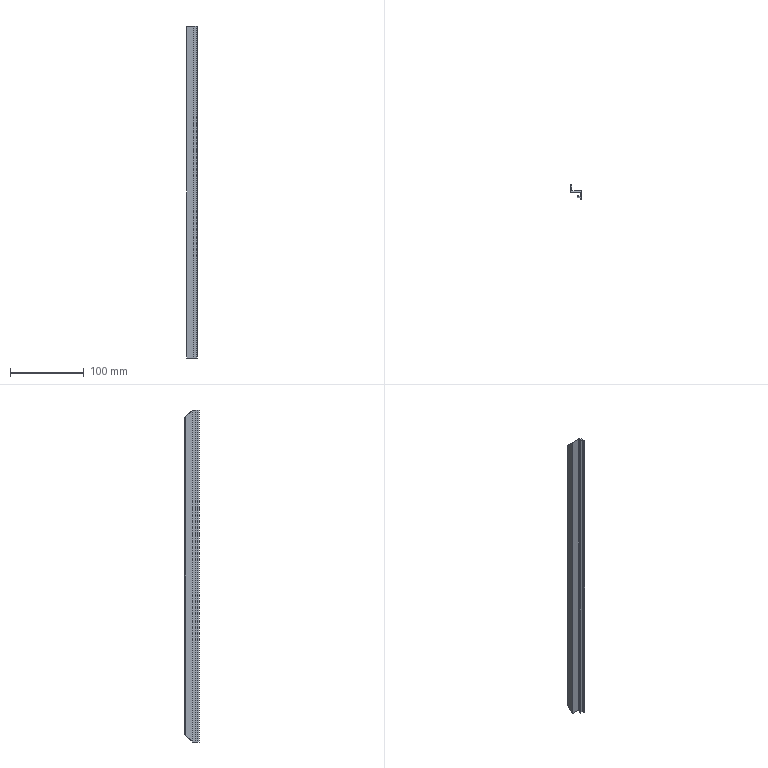Part | NX | features BREP 1 | 1 solid | 19 faces | box 14.9 x 19.1 x 450 mm | volume 31786 mm3 | plane 16 | cylinder 3 | commonest cylinder face diameters 1 x2 2 x1
STEP:
#1=CARTESIAN_POINT('',(12.9,-1.,223.5));
#2=VERTEX_POINT('',#1);
#3=CARTESIAN_POINT('',(12.9,-1.,-223.5));
#4=VERTEX_POINT('',#3);
#5=CARTESIAN_POINT('',(12.9,-1.,225.));
#6=DIRECTION('',(0.,0.,-1.));
#7=VECTOR('',#6,1000.);
#8=LINE('',#5,#7);
#9=EDGE_CURVE('',#2,#4,#8,.T.);
#10=ORIENTED_EDGE('',*,*,#9,.T.);
#11=CARTESIAN_POINT('',(12.4,-0.5,-223.));
#12=VERTEX_POINT('',#11);
#13=CARTESIAN_POINT('',(12.9,-1.,-223.5));
#14=CARTESIAN_POINT('',(12.9,-0.7071,-223.207));
#15=CARTESIAN_POINT('',(12.693,-0.5,-223.));
#16=CARTESIAN_POINT('',(12.4,-0.5,-223.));
#17=(BOUNDED_CURVE()B_SPLINE_CURVE(3,(#13,#14,#15,#16),.UNSPECIFIED.,.F.,.F.)B_SPLINE_CURVE_WITH_KNOTS((4,4),(1.571,3.142),.UNSPECIFIED.)CURVE()GEOMETRIC_REPRESENTATION_ITEM()RATIONAL_B_SPLINE_CURVE((1.,0.8047,0.8047,1.))REPRESENTATION_ITEM(''));
#18=EDGE_CURVE('',#4,#12,#17,.T.);
#19=ORIENTED_EDGE('',*,*,#18,.T.);
#20=CARTESIAN_POINT('',(12.4,-0.5,223.));
#21=VERTEX_POINT('',#20);
#22=CARTESIAN_POINT('',(12.4,-0.5,225.));
#23=DIRECTION('',(0.,0.,-1.));
#24=VECTOR('',#23,1000.);
#25=LINE('',#22,#24);
#26=EDGE_CURVE('',#21,#12,#25,.T.);
#27=ORIENTED_EDGE('',*,*,#26,.F.);
#28=CARTESIAN_POINT('',(12.4,-0.5,223.));
#29=CARTESIAN_POINT('',(12.693,-0.5,223.));
#30=CARTESIAN_POINT('',(12.9,-0.7071,223.207));
#31=CARTESIAN_POINT('',(12.9,-1.,223.5));
#32=(BOUNDED_CURVE()B_SPLINE_CURVE(3,(#28,#29,#30,#31),.UNSPECIFIED.,.F.,.F.)B_SPLINE_CURVE_WITH_KNOTS((4,4),(0.,1.571),.UNSPECIFIED.)CURVE()GEOMETRIC_REPRESENTATION_ITEM()RATIONAL_B_SPLINE_CURVE((1.,0.8047,0.8047,1.))REPRESENTATION_ITEM(''));
#33=EDGE_CURVE('',#21,#2,#32,.T.);
#34=ORIENTED_EDGE('',*,*,#33,.T.);
#35=EDGE_LOOP('',(#10,#19,#27,#34));
#36=FACE_BOUND('',#35,.T.);
#37=CARTESIAN_POINT('',(12.4,-1.,225.));
#38=DIRECTION('',(0.,0.,-1.));
#39=DIRECTION('',(-1.,0.,0.));
#40=AXIS2_PLACEMENT_3D('',#37,#38,#39);
#41=CYLINDRICAL_SURFACE('',#40,0.5);
#42=ADVANCED_FACE('',(#36),#41,.T.);
#43=ORIENTED_EDGE('',*,*,#26,.T.);
#44=CARTESIAN_POINT('',(0.,-0.5,-223.));
#45=VERTEX_POINT('',#44);
#46=CARTESIAN_POINT('',(0.,-0.5,-223.));
#47=DIRECTION('',(-1.,0.,0.));
#48=VECTOR('',#47,1000.);
#49=LINE('',#46,#48);
#50=EDGE_CURVE('',#12,#45,#49,.T.);
#51=ORIENTED_EDGE('',*,*,#50,.T.);
#52=CARTESIAN_POINT('',(0.,-0.5,223.));
#53=VERTEX_POINT('',#52);
#54=CARTESIAN_POINT('',(0.,-0.5,225.));
#55=DIRECTION('',(0.,0.,-1.));
#56=VECTOR('',#55,1000.);
#57=LINE('',#54,#56);
#58=EDGE_CURVE('',#53,#45,#57,.T.);
#59=ORIENTED_EDGE('',*,*,#58,.F.);
#60=CARTESIAN_POINT('',(12.4,-0.5,223.));
#61=DIRECTION('',(1.,0.,0.));
#62=VECTOR('',#61,1000.);
#63=LINE('',#60,#62);
#64=EDGE_CURVE('',#53,#21,#63,.T.);
#65=ORIENTED_EDGE('',*,*,#64,.T.);
#66=EDGE_LOOP('',(#43,#51,#59,#65));
#67=FACE_BOUND('',#66,.T.);
#68=CARTESIAN_POINT('',(12.4,-0.5,225.));
#69=DIRECTION('',(0.,-1.,0.));
#70=DIRECTION('',(0.,0.,-1.));
#71=AXIS2_PLACEMENT_3D('',#68,#69,#70);
#72=PLANE('',#71);
#73=ADVANCED_FACE('',(#67),#72,.F.);
#74=ORIENTED_EDGE('',*,*,#58,.T.);
#75=CARTESIAN_POINT('',(0.,7.5,-215.));
#76=VERTEX_POINT('',#75);
#77=CARTESIAN_POINT('',(0.,7.5,-215.));
#78=DIRECTION('',(0.,0.7071,0.7071));
#79=VECTOR('',#78,1000.);
#80=LINE('',#77,#79);
#81=EDGE_CURVE('',#45,#76,#80,.T.);
#82=ORIENTED_EDGE('',*,*,#81,.T.);
#83=CARTESIAN_POINT('',(0.,7.5,215.));
#84=VERTEX_POINT('',#83);
#85=CARTESIAN_POINT('',(0.,7.5,225.));
#86=DIRECTION('',(0.,0.,-1.));
#87=VECTOR('',#86,1000.);
#88=LINE('',#85,#87);
#89=EDGE_CURVE('',#84,#76,#88,.T.);
#90=ORIENTED_EDGE('',*,*,#89,.F.);
#91=CARTESIAN_POINT('',(0.,-2.5,225.));
#92=DIRECTION('',(0.,-0.7071,0.7071));
#93=VECTOR('',#92,1000.);
#94=LINE('',#91,#93);
#95=EDGE_CURVE('',#84,#53,#94,.T.);
#96=ORIENTED_EDGE('',*,*,#95,.T.);
#97=EDGE_LOOP('',(#74,#82,#90,#96));
#98=FACE_BOUND('',#97,.T.);
#99=CARTESIAN_POINT('',(0.,-0.5,225.));
#100=DIRECTION('',(-1.,0.,0.));
#101=DIRECTION('',(0.,0.,1.));
#102=AXIS2_PLACEMENT_3D('',#99,#100,#101);
#103=PLANE('',#102);
#104=ADVANCED_FACE('',(#98),#103,.F.);
#105=ORIENTED_EDGE('',*,*,#89,.T.);
#106=CARTESIAN_POINT('',(-1.,7.5,-215.));
#107=VERTEX_POINT('',#106);
#108=CARTESIAN_POINT('',(0.,7.5,-215.));
#109=DIRECTION('',(-1.,0.,0.));
#110=VECTOR('',#109,1000.);
#111=LINE('',#108,#110);
#112=EDGE_CURVE('',#76,#107,#111,.T.);
#113=ORIENTED_EDGE('',*,*,#112,.T.);
#114=CARTESIAN_POINT('',(-1.,7.5,215.));
#115=VERTEX_POINT('',#114);
#116=CARTESIAN_POINT('',(-1.,7.5,225.));
#117=DIRECTION('',(0.,0.,-1.));
#118=VECTOR('',#117,1000.);
#119=LINE('',#116,#118);
#120=EDGE_CURVE('',#115,#107,#119,.T.);
#121=ORIENTED_EDGE('',*,*,#120,.F.);
#122=CARTESIAN_POINT('',(0.,7.5,215.));
#123=DIRECTION('',(1.,0.,0.));
#124=VECTOR('',#123,1000.);
#125=LINE('',#122,#124);
#126=EDGE_CURVE('',#115,#84,#125,.T.);
#127=ORIENTED_EDGE('',*,*,#126,.T.);
#128=EDGE_LOOP('',(#105,#113,#121,#127));
#129=FACE_BOUND('',#128,.T.);
#130=CARTESIAN_POINT('',(0.,7.5,225.));
#131=DIRECTION('',(0.,-1.,0.));
#132=DIRECTION('',(0.,0.,-1.));
#133=AXIS2_PLACEMENT_3D('',#130,#131,#132);
#134=PLANE('',#133);
#135=ADVANCED_FACE('',(#129),#134,.F.);
#136=ORIENTED_EDGE('',*,*,#120,.T.);
#137=CARTESIAN_POINT('',(-2.,6.5,-216.));
#138=VERTEX_POINT('',#137);
#139=CARTESIAN_POINT('',(-1.,7.5,-215.));
#140=CARTESIAN_POINT('',(-1.586,7.5,-215.));
#141=CARTESIAN_POINT('',(-2.,7.086,-215.414));
#142=CARTESIAN_POINT('',(-2.,6.5,-216.));
#143=(BOUNDED_CURVE()B_SPLINE_CURVE(3,(#139,#140,#141,#142),.UNSPECIFIED.,.F.,.F.)B_SPLINE_CURVE_WITH_KNOTS((4,4),(3.142,4.712),.UNSPECIFIED.)CURVE()GEOMETRIC_REPRESENTATION_ITEM()RATIONAL_B_SPLINE_CURVE((1.,0.8047,0.8047,1.))REPRESENTATION_ITEM(''));
#144=EDGE_CURVE('',#107,#138,#143,.T.);
#145=ORIENTED_EDGE('',*,*,#144,.T.);
#146=CARTESIAN_POINT('',(-2.,6.5,216.));
#147=VERTEX_POINT('',#146);
#148=CARTESIAN_POINT('',(-2.,6.5,225.));
#149=DIRECTION('',(0.,0.,-1.));
#150=VECTOR('',#149,1000.);
#151=LINE('',#148,#150);
#152=EDGE_CURVE('',#147,#138,#151,.T.);
#153=ORIENTED_EDGE('',*,*,#152,.F.);
#154=CARTESIAN_POINT('',(-2.,6.5,216.));
#155=CARTESIAN_POINT('',(-2.,7.086,215.414));
#156=CARTESIAN_POINT('',(-1.586,7.5,215.));
#157=CARTESIAN_POINT('',(-1.,7.5,215.));
#158=(BOUNDED_CURVE()B_SPLINE_CURVE(3,(#154,#155,#156,#157),.UNSPECIFIED.,.F.,.F.)B_SPLINE_CURVE_WITH_KNOTS((4,4),(4.712,6.283),.UNSPECIFIED.)CURVE()GEOMETRIC_REPRESENTATION_ITEM()RATIONAL_B_SPLINE_CURVE((1.,0.8047,0.8047,1.))REPRESENTATION_ITEM(''));
#159=EDGE_CURVE('',#147,#115,#158,.T.);
#160=ORIENTED_EDGE('',*,*,#159,.T.);
#161=EDGE_LOOP('',(#136,#145,#153,#160));
#162=FACE_BOUND('',#161,.T.);
#163=CARTESIAN_POINT('',(-1.,6.5,225.));
#164=DIRECTION('',(0.,0.,-1.));
#165=DIRECTION('',(-1.,0.,0.));
#166=AXIS2_PLACEMENT_3D('',#163,#164,#165);
#167=CYLINDRICAL_SURFACE('',#166,1.);
#168=ADVANCED_FACE('',(#162),#167,.T.);
#169=ORIENTED_EDGE('',*,*,#152,.T.);
#170=CARTESIAN_POINT('',(-2.,-2.5,-225.));
#171=VERTEX_POINT('',#170);
#172=CARTESIAN_POINT('',(-2.,7.5,-215.));
#173=DIRECTION('',(0.,-0.7071,-0.7071));
#174=VECTOR('',#173,1000.);
#175=LINE('',#172,#174);
#176=EDGE_CURVE('',#138,#171,#175,.T.);
#177=ORIENTED_EDGE('',*,*,#176,.T.);
#178=CARTESIAN_POINT('',(-2.,-2.5,225.));
#179=VERTEX_POINT('',#178);
#180=CARTESIAN_POINT('',(-2.,-2.5,225.));
#181=DIRECTION('',(0.,0.,-1.));
#182=VECTOR('',#181,1000.);
#183=LINE('',#180,#182);
#184=EDGE_CURVE('',#179,#171,#183,.T.);
#185=ORIENTED_EDGE('',*,*,#184,.F.);
#186=CARTESIAN_POINT('',(-2.,-2.5,225.));
#187=DIRECTION('',(0.,0.7071,-0.7071));
#188=VECTOR('',#187,1000.);
#189=LINE('',#186,#188);
#190=EDGE_CURVE('',#179,#147,#189,.T.);
#191=ORIENTED_EDGE('',*,*,#190,.T.);
#192=EDGE_LOOP('',(#169,#177,#185,#191));
#193=FACE_BOUND('',#192,.T.);
#194=CARTESIAN_POINT('',(-2.,6.5,225.));
#195=DIRECTION('',(1.,0.,0.));
#196=DIRECTION('',(0.,1.,0.));
#197=AXIS2_PLACEMENT_3D('',#194,#195,#196);
#198=PLANE('',#197);
#199=ADVANCED_FACE('',(#193),#198,.F.);
#200=CARTESIAN_POINT('',(10.4,-2.5,-225.));
#201=VERTEX_POINT('',#200);
#202=CARTESIAN_POINT('',(-2.,-2.5,-225.));
#203=DIRECTION('',(1.,0.,0.));
#204=VECTOR('',#203,1000.);
#205=LINE('',#202,#204);
#206=EDGE_CURVE('',#171,#201,#205,.T.);
#207=ORIENTED_EDGE('',*,*,#206,.T.);
#208=CARTESIAN_POINT('',(10.4,-2.5,225.));
#209=VERTEX_POINT('',#208);
#210=CARTESIAN_POINT('',(10.4,-2.5,225.));
#211=DIRECTION('',(0.,0.,-1.));
#212=VECTOR('',#211,1000.);
#213=LINE('',#210,#212);
#214=EDGE_CURVE('',#209,#201,#213,.T.);
#215=ORIENTED_EDGE('',*,*,#214,.F.);
#216=CARTESIAN_POINT('',(-2.,-2.5,225.));
#217=DIRECTION('',(1.,0.,0.));
#218=VECTOR('',#217,1000.);
#219=LINE('',#216,#218);
#220=EDGE_CURVE('',#179,#209,#219,.T.);
#221=ORIENTED_EDGE('',*,*,#220,.F.);
#222=ORIENTED_EDGE('',*,*,#184,.T.);
#223=EDGE_LOOP('',(#207,#215,#221,#222));
#224=FACE_BOUND('',#223,.T.);
#225=CARTESIAN_POINT('',(-2.,-2.5,225.));
#226=DIRECTION('',(0.,1.,0.));
#227=DIRECTION('',(1.,0.,0.));
#228=AXIS2_PLACEMENT_3D('',#225,#226,#227);
#229=PLANE('',#228);
#230=ADVANCED_FACE('',(#224),#229,.F.);
#231=CARTESIAN_POINT('',(10.9,-3.,-225.));
#232=VERTEX_POINT('',#231);
#233=CARTESIAN_POINT('',(10.4,-3.,-225.));
#234=DIRECTION('',(0.,0.,-1.));
#235=DIRECTION('',(1.,0.,0.));
#236=AXIS2_PLACEMENT_3D('',#233,#234,#235);
#237=CIRCLE('',#236,0.5);
#238=EDGE_CURVE('',#201,#232,#237,.T.);
#239=ORIENTED_EDGE('',*,*,#238,.T.);
#240=CARTESIAN_POINT('',(10.9,-3.,225.));
#241=VERTEX_POINT('',#240);
#242=CARTESIAN_POINT('',(10.9,-3.,225.));
#243=DIRECTION('',(0.,0.,-1.));
#244=VECTOR('',#243,1000.);
#245=LINE('',#242,#244);
#246=EDGE_CURVE('',#241,#232,#245,.T.);
#247=ORIENTED_EDGE('',*,*,#246,.F.);
#248=CARTESIAN_POINT('',(10.4,-3.,225.));
#249=DIRECTION('',(0.,0.,-1.));
#250=DIRECTION('',(1.,0.,0.));
#251=AXIS2_PLACEMENT_3D('',#248,#249,#250);
#252=CIRCLE('',#251,0.5);
#253=EDGE_CURVE('',#209,#241,#252,.T.);
#254=ORIENTED_EDGE('',*,*,#253,.F.);
#255=ORIENTED_EDGE('',*,*,#214,.T.);
#256=EDGE_LOOP('',(#239,#247,#254,#255));
#257=FACE_BOUND('',#256,.T.);
#258=CARTESIAN_POINT('',(10.4,-3.,225.));
#259=DIRECTION('',(0.,0.,-1.));
#260=DIRECTION('',(-1.,0.,0.));
#261=AXIS2_PLACEMENT_3D('',#258,#259,#260);
#262=CYLINDRICAL_SURFACE('',#261,0.5);
#263=ADVANCED_FACE('',(#257),#262,.F.);
#264=CARTESIAN_POINT('',(10.9,-7.2,-225.));
#265=VERTEX_POINT('',#264);
#266=CARTESIAN_POINT('',(10.9,-3.,-225.));
#267=DIRECTION('',(0.,-1.,0.));
#268=VECTOR('',#267,1000.);
#269=LINE('',#266,#268);
#270=EDGE_CURVE('',#232,#265,#269,.T.);
#271=ORIENTED_EDGE('',*,*,#270,.T.);
#272=CARTESIAN_POINT('',(10.9,-7.2,225.));
#273=VERTEX_POINT('',#272);
#274=CARTESIAN_POINT('',(10.9,-7.2,225.));
#275=DIRECTION('',(0.,0.,-1.));
#276=VECTOR('',#275,1000.);
#277=LINE('',#274,#276);
#278=EDGE_CURVE('',#273,#265,#277,.T.);
#279=ORIENTED_EDGE('',*,*,#278,.F.);
#280=CARTESIAN_POINT('',(10.9,-3.,225.));
#281=DIRECTION('',(0.,-1.,0.));
#282=VECTOR('',#281,1000.);
#283=LINE('',#280,#282);
#284=EDGE_CURVE('',#241,#273,#283,.T.);
#285=ORIENTED_EDGE('',*,*,#284,.F.);
#286=ORIENTED_EDGE('',*,*,#246,.T.);
#287=EDGE_LOOP('',(#271,#279,#285,#286));
#288=FACE_BOUND('',#287,.T.);
#289=CARTESIAN_POINT('',(10.9,-3.,225.));
#290=DIRECTION('',(1.,0.,0.));
#291=DIRECTION('',(0.,1.,0.));
#292=AXIS2_PLACEMENT_3D('',#289,#290,#291);
#293=PLANE('',#292);
#294=ADVANCED_FACE('',(#288),#293,.F.);
#295=CARTESIAN_POINT('',(7.2,-7.2,-225.));
#296=VERTEX_POINT('',#295);
#297=CARTESIAN_POINT('',(10.9,-7.2,-225.));
#298=DIRECTION('',(-1.,0.,0.));
#299=VECTOR('',#298,1000.);
#300=LINE('',#297,#299);
#301=EDGE_CURVE('',#265,#296,#300,.T.);
#302=ORIENTED_EDGE('',*,*,#301,.T.);
#303=CARTESIAN_POINT('',(7.2,-7.2,225.));
#304=VERTEX_POINT('',#303);
#305=CARTESIAN_POINT('',(7.2,-7.2,225.));
#306=DIRECTION('',(0.,0.,-1.));
#307=VECTOR('',#306,1000.);
#308=LINE('',#305,#307);
#309=EDGE_CURVE('',#304,#296,#308,.T.);
#310=ORIENTED_EDGE('',*,*,#309,.F.);
#311=CARTESIAN_POINT('',(10.9,-7.2,225.));
#312=DIRECTION('',(-1.,0.,0.));
#313=VECTOR('',#312,1000.);
#314=LINE('',#311,#313);
#315=EDGE_CURVE('',#273,#304,#314,.T.);
#316=ORIENTED_EDGE('',*,*,#315,.F.);
#317=ORIENTED_EDGE('',*,*,#278,.T.);
#318=EDGE_LOOP('',(#302,#310,#316,#317));
#319=FACE_BOUND('',#318,.T.);
#320=CARTESIAN_POINT('',(10.9,-7.2,225.));
#321=DIRECTION('',(0.,-1.,0.));
#322=DIRECTION('',(0.,0.,-1.));
#323=AXIS2_PLACEMENT_3D('',#320,#321,#322);
#324=PLANE('',#323);
#325=ADVANCED_FACE('',(#319),#324,.F.);
#326=CARTESIAN_POINT('',(7.2,-9.2,-225.));
#327=VERTEX_POINT('',#326);
#328=CARTESIAN_POINT('',(7.2,-7.2,-225.));
#329=DIRECTION('',(0.,-1.,0.));
#330=VECTOR('',#329,1000.);
#331=LINE('',#328,#330);
#332=EDGE_CURVE('',#296,#327,#331,.T.);
#333=ORIENTED_EDGE('',*,*,#332,.T.);
#334=CARTESIAN_POINT('',(7.2,-9.2,225.));
#335=VERTEX_POINT('',#334);
#336=CARTESIAN_POINT('',(7.2,-9.2,225.));
#337=DIRECTION('',(0.,0.,-1.));
#338=VECTOR('',#337,1000.);
#339=LINE('',#336,#338);
#340=EDGE_CURVE('',#335,#327,#339,.T.);
#341=ORIENTED_EDGE('',*,*,#340,.F.);
#342=CARTESIAN_POINT('',(7.2,-7.2,225.));
#343=DIRECTION('',(0.,-1.,0.));
#344=VECTOR('',#343,1000.);
#345=LINE('',#342,#344);
#346=EDGE_CURVE('',#304,#335,#345,.T.);
#347=ORIENTED_EDGE('',*,*,#346,.F.);
#348=ORIENTED_EDGE('',*,*,#309,.T.);
#349=EDGE_LOOP('',(#333,#341,#347,#348));
#350=FACE_BOUND('',#349,.T.);
#351=CARTESIAN_POINT('',(7.2,-7.2,225.));
#352=DIRECTION('',(1.,0.,0.));
#353=DIRECTION('',(0.,1.,0.));
#354=AXIS2_PLACEMENT_3D('',#351,#352,#353);
#355=PLANE('',#354);
#356=ADVANCED_FACE('',(#350),#355,.F.);
#357=CARTESIAN_POINT('',(10.9,-9.2,-225.));
#358=VERTEX_POINT('',#357);
#359=CARTESIAN_POINT('',(7.2,-9.2,-225.));
#360=DIRECTION('',(1.,0.,0.));
#361=VECTOR('',#360,1000.);
#362=LINE('',#359,#361);
#363=EDGE_CURVE('',#327,#358,#362,.T.);
#364=ORIENTED_EDGE('',*,*,#363,.T.);
#365=CARTESIAN_POINT('',(10.9,-9.2,225.));
#366=VERTEX_POINT('',#365);
#367=CARTESIAN_POINT('',(10.9,-9.2,225.));
#368=DIRECTION('',(0.,0.,-1.));
#369=VECTOR('',#368,1000.);
#370=LINE('',#367,#369);
#371=EDGE_CURVE('',#366,#358,#370,.T.);
#372=ORIENTED_EDGE('',*,*,#371,.F.);
#373=CARTESIAN_POINT('',(7.2,-9.2,225.));
#374=DIRECTION('',(1.,0.,0.));
#375=VECTOR('',#374,1000.);
#376=LINE('',#373,#375);
#377=EDGE_CURVE('',#335,#366,#376,.T.);
#378=ORIENTED_EDGE('',*,*,#377,.F.);
#379=ORIENTED_EDGE('',*,*,#340,.T.);
#380=EDGE_LOOP('',(#364,#372,#378,#379));
#381=FACE_BOUND('',#380,.T.);
#382=CARTESIAN_POINT('',(7.2,-9.2,225.));
#383=DIRECTION('',(0.,1.,0.));
#384=DIRECTION('',(1.,0.,0.));
#385=AXIS2_PLACEMENT_3D('',#382,#383,#384);
#386=PLANE('',#385);
#387=ADVANCED_FACE('',(#381),#386,.F.);
#388=CARTESIAN_POINT('',(10.9,-11.6,-225.));
#389=VERTEX_POINT('',#388);
#390=CARTESIAN_POINT('',(10.9,-9.2,-225.));
#391=DIRECTION('',(0.,-1.,0.));
#392=VECTOR('',#391,1000.);
#393=LINE('',#390,#392);
#394=EDGE_CURVE('',#358,#389,#393,.T.);
#395=ORIENTED_EDGE('',*,*,#394,.T.);
#396=CARTESIAN_POINT('',(10.9,-11.6,225.));
#397=VERTEX_POINT('',#396);
#398=CARTESIAN_POINT('',(10.9,-11.6,225.));
#399=DIRECTION('',(0.,0.,-1.));
#400=VECTOR('',#399,1000.);
#401=LINE('',#398,#400);
#402=EDGE_CURVE('',#397,#389,#401,.T.);
#403=ORIENTED_EDGE('',*,*,#402,.F.);
#404=CARTESIAN_POINT('',(10.9,-9.2,225.));
#405=DIRECTION('',(0.,-1.,0.));
#406=VECTOR('',#405,1000.);
#407=LINE('',#404,#406);
#408=EDGE_CURVE('',#366,#397,#407,.T.);
#409=ORIENTED_EDGE('',*,*,#408,.F.);
#410=ORIENTED_EDGE('',*,*,#371,.T.);
#411=EDGE_LOOP('',(#395,#403,#409,#410));
#412=FACE_BOUND('',#411,.T.);
#413=CARTESIAN_POINT('',(10.9,-9.2,225.));
#414=DIRECTION('',(1.,0.,0.));
#415=DIRECTION('',(0.,1.,0.));
#416=AXIS2_PLACEMENT_3D('',#413,#414,#415);
#417=PLANE('',#416);
#418=ADVANCED_FACE('',(#412),#417,.F.);
#419=CARTESIAN_POINT('',(12.9,-11.6,-225.));
#420=VERTEX_POINT('',#419);
#421=CARTESIAN_POINT('',(10.9,-11.6,-225.));
#422=DIRECTION('',(1.,0.,0.));
#423=VECTOR('',#422,1000.);
#424=LINE('',#421,#423);
#425=EDGE_CURVE('',#389,#420,#424,.T.);
#426=ORIENTED_EDGE('',*,*,#425,.T.);
#427=CARTESIAN_POINT('',(12.9,-11.6,225.));
#428=VERTEX_POINT('',#427);
#429=CARTESIAN_POINT('',(12.9,-11.6,225.));
#430=DIRECTION('',(0.,0.,-1.));
#431=VECTOR('',#430,1000.);
#432=LINE('',#429,#431);
#433=EDGE_CURVE('',#428,#420,#432,.T.);
#434=ORIENTED_EDGE('',*,*,#433,.F.);
#435=CARTESIAN_POINT('',(10.9,-11.6,225.));
#436=DIRECTION('',(1.,0.,0.));
#437=VECTOR('',#436,1000.);
#438=LINE('',#435,#437);
#439=EDGE_CURVE('',#397,#428,#438,.T.);
#440=ORIENTED_EDGE('',*,*,#439,.F.);
#441=ORIENTED_EDGE('',*,*,#402,.T.);
#442=EDGE_LOOP('',(#426,#434,#440,#441));
#443=FACE_BOUND('',#442,.T.);
#444=CARTESIAN_POINT('',(10.9,-11.6,225.));
#445=DIRECTION('',(0.,1.,0.));
#446=DIRECTION('',(1.,0.,0.));
#447=AXIS2_PLACEMENT_3D('',#444,#445,#446);
#448=PLANE('',#447);
#449=ADVANCED_FACE('',(#443),#448,.F.);
#450=CARTESIAN_POINT('',(12.9,-2.5,-225.));
#451=VERTEX_POINT('',#450);
#452=CARTESIAN_POINT('',(12.9,-11.6,-225.));
#453=DIRECTION('',(0.,1.,0.));
#454=VECTOR('',#453,1000.);
#455=LINE('',#452,#454);
#456=EDGE_CURVE('',#420,#451,#455,.T.);
#457=ORIENTED_EDGE('',*,*,#456,.T.);
#458=CARTESIAN_POINT('',(12.9,7.5,-215.));
#459=DIRECTION('',(0.,0.7071,0.7071));
#460=VECTOR('',#459,1000.);
#461=LINE('',#458,#460);
#462=EDGE_CURVE('',#451,#4,#461,.T.);
#463=ORIENTED_EDGE('',*,*,#462,.T.);
#464=ORIENTED_EDGE('',*,*,#9,.F.);
#465=CARTESIAN_POINT('',(12.9,-2.5,225.));
#466=VERTEX_POINT('',#465);
#467=CARTESIAN_POINT('',(12.9,-2.5,225.));
#468=DIRECTION('',(0.,-0.7071,0.7071));
#469=VECTOR('',#468,1000.);
#470=LINE('',#467,#469);
#471=EDGE_CURVE('',#2,#466,#470,.T.);
#472=ORIENTED_EDGE('',*,*,#471,.T.);
#473=CARTESIAN_POINT('',(12.9,-11.6,225.));
#474=DIRECTION('',(0.,1.,0.));
#475=VECTOR('',#474,1000.);
#476=LINE('',#473,#475);
#477=EDGE_CURVE('',#428,#466,#476,.T.);
#478=ORIENTED_EDGE('',*,*,#477,.F.);
#479=ORIENTED_EDGE('',*,*,#433,.T.);
#480=EDGE_LOOP('',(#457,#463,#464,#472,#478,#479));
#481=FACE_BOUND('',#480,.T.);
#482=CARTESIAN_POINT('',(12.9,-11.6,225.));
#483=DIRECTION('',(-1.,0.,0.));
#484=DIRECTION('',(0.,1.,0.));
#485=AXIS2_PLACEMENT_3D('',#482,#483,#484);
#486=PLANE('',#485);
#487=ADVANCED_FACE('',(#481),#486,.F.);
#488=ORIENTED_EDGE('',*,*,#477,.T.);
#489=CARTESIAN_POINT('',(-1.,-2.5,225.));
#490=DIRECTION('',(-1.,0.,0.));
#491=VECTOR('',#490,1000.);
#492=LINE('',#489,#491);
#493=EDGE_CURVE('',#466,#209,#492,.T.);
#494=ORIENTED_EDGE('',*,*,#493,.T.);
#495=ORIENTED_EDGE('',*,*,#253,.T.);
#496=ORIENTED_EDGE('',*,*,#284,.T.);
#497=ORIENTED_EDGE('',*,*,#315,.T.);
#498=ORIENTED_EDGE('',*,*,#346,.T.);
#499=ORIENTED_EDGE('',*,*,#377,.T.);
#500=ORIENTED_EDGE('',*,*,#408,.T.);
#501=ORIENTED_EDGE('',*,*,#439,.T.);
#502=EDGE_LOOP('',(#488,#494,#495,#496,#497,#498,#499,#500,#501));
#503=FACE_BOUND('',#502,.T.);
#504=CARTESIAN_POINT('',(12.4,-1.,225.));
#505=DIRECTION('',(0.,0.,1.));
#506=DIRECTION('',(1.,0.,0.));
#507=AXIS2_PLACEMENT_3D('',#504,#505,#506);
#508=PLANE('',#507);
#509=ADVANCED_FACE('',(#503),#508,.T.);
#510=ORIENTED_EDGE('',*,*,#238,.F.);
#511=CARTESIAN_POINT('',(12.4,-2.5,-225.));
#512=DIRECTION('',(1.,0.,0.));
#513=VECTOR('',#512,1000.);
#514=LINE('',#511,#513);
#515=EDGE_CURVE('',#201,#451,#514,.T.);
#516=ORIENTED_EDGE('',*,*,#515,.T.);
#517=ORIENTED_EDGE('',*,*,#456,.F.);
#518=ORIENTED_EDGE('',*,*,#425,.F.);
#519=ORIENTED_EDGE('',*,*,#394,.F.);
#520=ORIENTED_EDGE('',*,*,#363,.F.);
#521=ORIENTED_EDGE('',*,*,#332,.F.);
#522=ORIENTED_EDGE('',*,*,#301,.F.);
#523=ORIENTED_EDGE('',*,*,#270,.F.);
#524=EDGE_LOOP('',(#510,#516,#517,#518,#519,#520,#521,#522,#523));
#525=FACE_BOUND('',#524,.T.);
#526=CARTESIAN_POINT('',(12.4,-1.,-225.));
#527=DIRECTION('',(0.,0.,1.));
#528=DIRECTION('',(1.,0.,0.));
#529=AXIS2_PLACEMENT_3D('',#526,#527,#528);
#530=PLANE('',#529);
#531=ADVANCED_FACE('',(#525),#530,.F.);
#532=ORIENTED_EDGE('',*,*,#515,.F.);
#533=ORIENTED_EDGE('',*,*,#206,.F.);
#534=ORIENTED_EDGE('',*,*,#176,.F.);
#535=ORIENTED_EDGE('',*,*,#144,.F.);
#536=ORIENTED_EDGE('',*,*,#112,.F.);
#537=ORIENTED_EDGE('',*,*,#81,.F.);
#538=ORIENTED_EDGE('',*,*,#50,.F.);
#539=ORIENTED_EDGE('',*,*,#18,.F.);
#540=ORIENTED_EDGE('',*,*,#462,.F.);
#541=EDGE_LOOP('',(#532,#533,#534,#535,#536,#537,#538,#539,#540));
#542=FACE_BOUND('',#541,.T.);
#543=CARTESIAN_POINT('',(0.,7.5,-215.));
#544=DIRECTION('',(0.,-0.7071,0.7071));
#545=DIRECTION('',(-1.,0.,0.));
#546=AXIS2_PLACEMENT_3D('',#543,#544,#545);
#547=PLANE('',#546);
#548=ADVANCED_FACE('',(#542),#547,.F.);
#549=ORIENTED_EDGE('',*,*,#95,.F.);
#550=ORIENTED_EDGE('',*,*,#126,.F.);
#551=ORIENTED_EDGE('',*,*,#159,.F.);
#552=ORIENTED_EDGE('',*,*,#190,.F.);
#553=ORIENTED_EDGE('',*,*,#220,.T.);
#554=ORIENTED_EDGE('',*,*,#493,.F.);
#555=ORIENTED_EDGE('',*,*,#471,.F.);
#556=ORIENTED_EDGE('',*,*,#33,.F.);
#557=ORIENTED_EDGE('',*,*,#64,.F.);
#558=EDGE_LOOP('',(#549,#550,#551,#552,#553,#554,#555,#556,#557));
#559=FACE_BOUND('',#558,.T.);
#560=CARTESIAN_POINT('',(12.4,-2.5,225.));
#561=DIRECTION('',(0.,0.7071,0.7071));
#562=DIRECTION('',(1.,0.,0.));
#563=AXIS2_PLACEMENT_3D('',#560,#561,#562);
#564=PLANE('',#563);
#565=ADVANCED_FACE('',(#559),#564,.T.);
#566=CLOSED_SHELL('',(#42,#73,#104,#135,#168,#199,#230,#263,#294,#325,#356,#387,#418,#449,#487,#509,#531,#548,#565));
#567=MANIFOLD_SOLID_BREP('',#566);
#568=(LENGTH_UNIT()NAMED_UNIT(*)SI_UNIT(.MILLI.,.METRE.));
#569=UNCERTAINTY_MEASURE_WITH_UNIT(LENGTH_MEASURE(0.00001),#568,'','');
#570=(NAMED_UNIT(*)PLANE_ANGLE_UNIT()SI_UNIT($,.RADIAN.));
#571=(NAMED_UNIT(*)SI_UNIT($,.STERADIAN.)SOLID_ANGLE_UNIT());
#572=(GEOMETRIC_REPRESENTATION_CONTEXT(3)GLOBAL_UNCERTAINTY_ASSIGNED_CONTEXT((#569))GLOBAL_UNIT_ASSIGNED_CONTEXT((#568,#570,#571))REPRESENTATION_CONTEXT('',''));
#573=ADVANCED_BREP_SHAPE_REPRESENTATION('',(#567),#572);